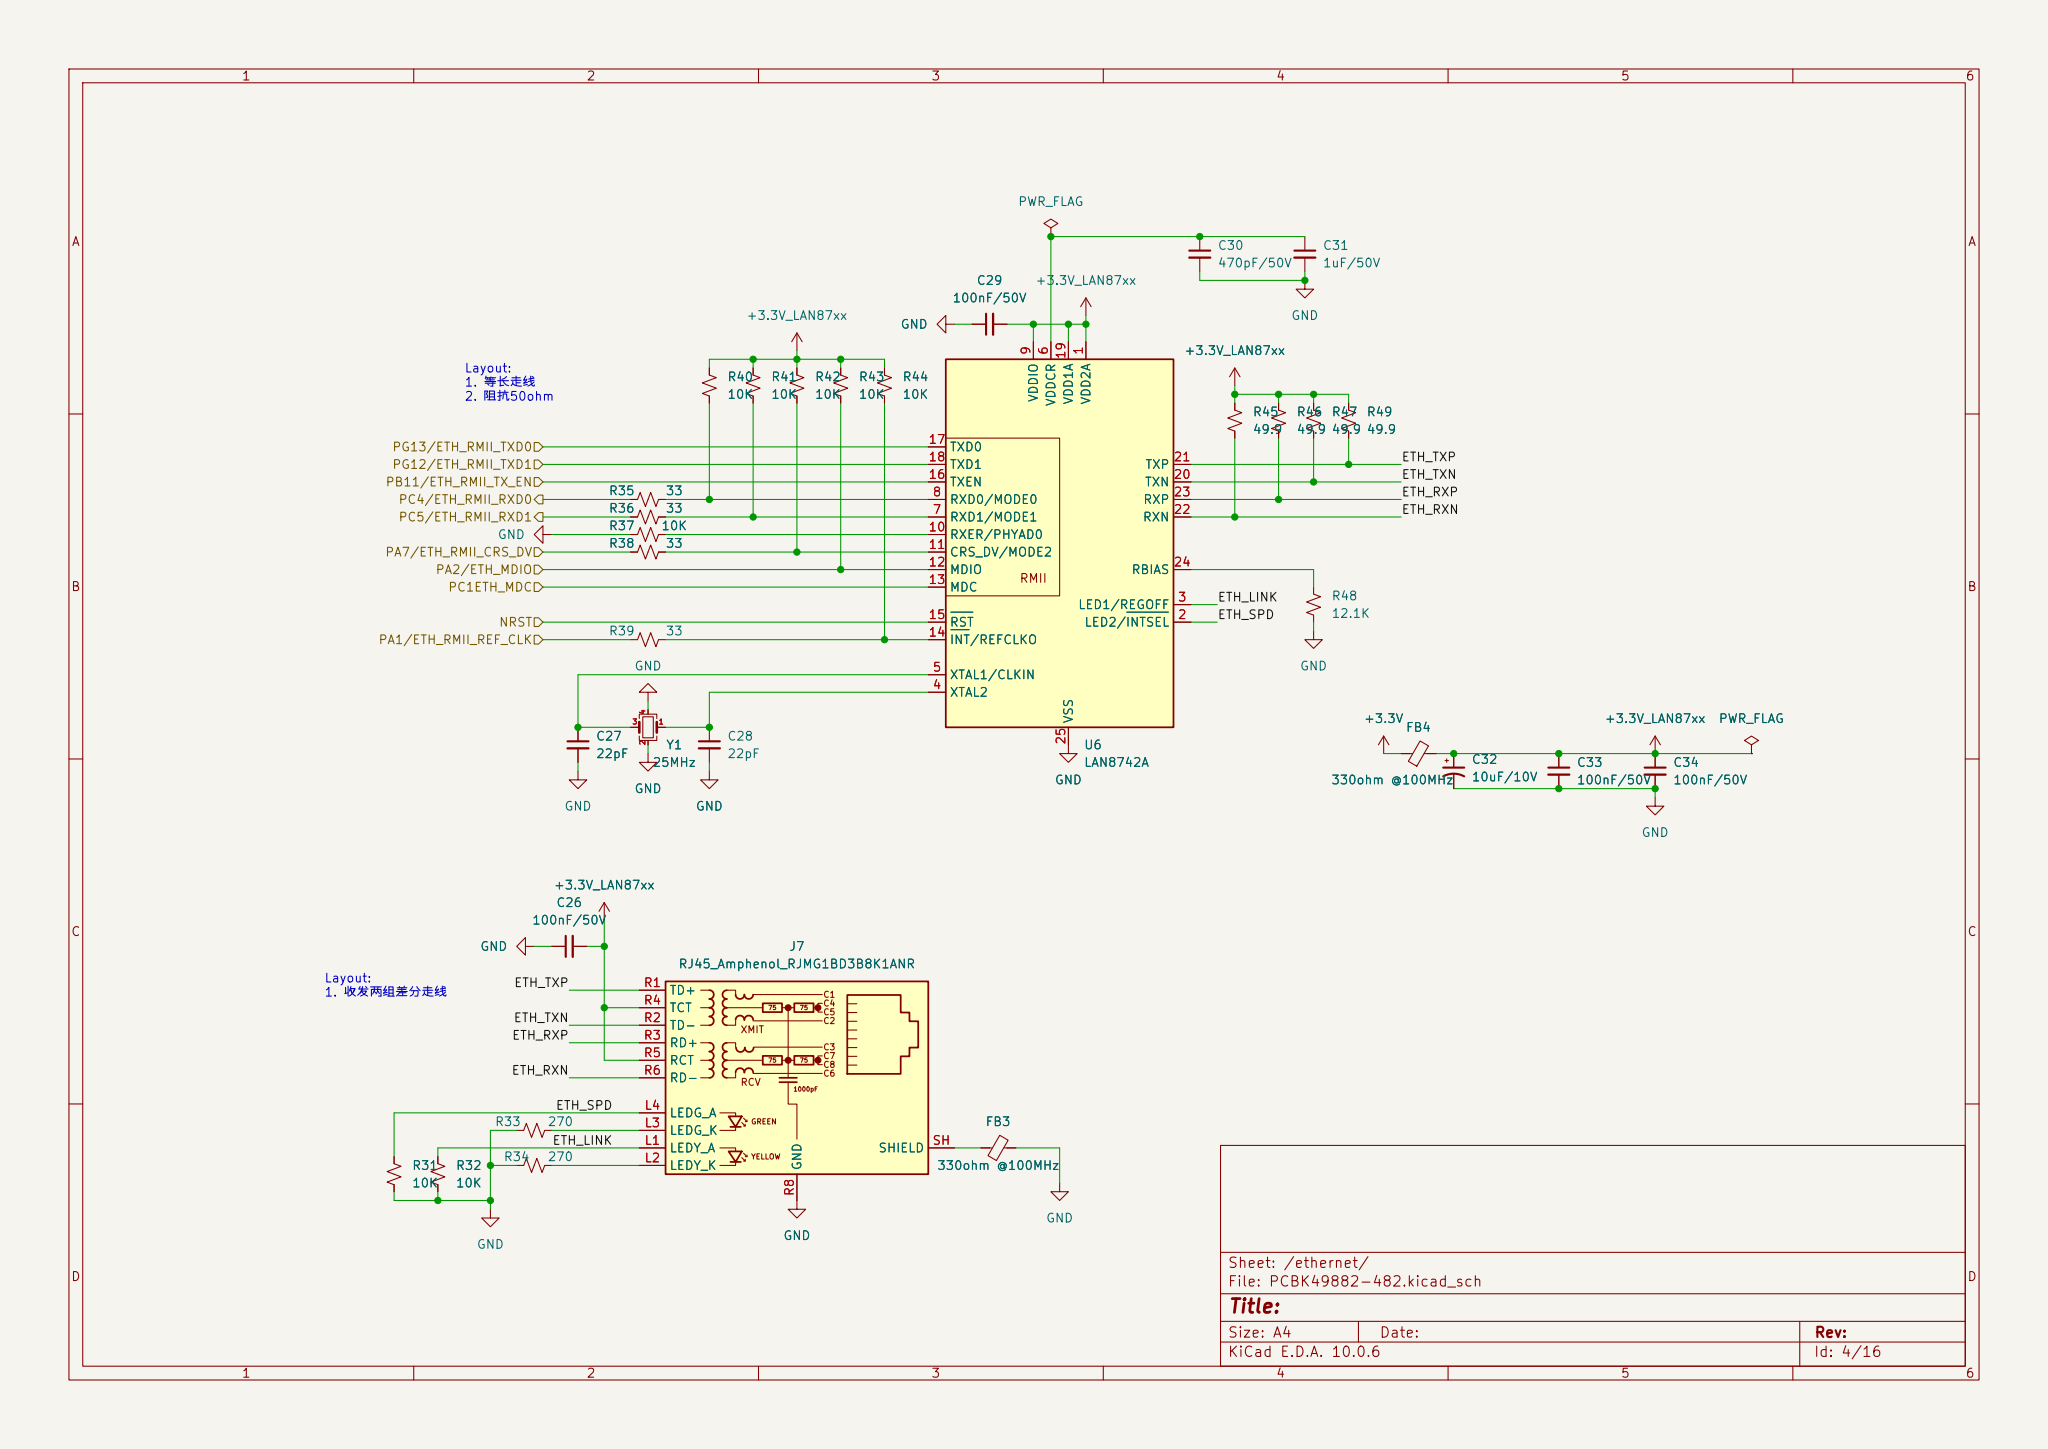Circuit board | KiCad | 536 parts | 438 nets | one sheet of the schematic
Parts on this sheet (reference | value | footprint):
C26 | 100nF/50V | Capacitor_SMD:C_0603_1608Metric
C27 | 22pF | Capacitor_SMD:C_0603_1608Metric
C28 | 22pF | Capacitor_SMD:C_0603_1608Metric
C29 | 100nF/50V | Capacitor_SMD:C_0603_1608Metric
C30 | 470pF/50V | Capacitor_SMD:C_0603_1608Metric
C31 | 1uF/50V | Capacitor_SMD:C_0603_1608Metric
C32 | 10uF/10V | Capacitor_Tantalum_SMD:CP_EIA-3528-21_Kemet-B
C33 | 100nF/50V | Capacitor_SMD:C_0603_1608Metric
C34 | 100nF/50V | Capacitor_SMD:C_0603_1608Metric
FB3
FB4
J7 | RJ45_Amphenol_RJMG1BD3B8K1ANR | Connector_RJ:RJ45_Amphenol_RJMG1BD3B8K1ANR
R31
R32
R33 | 270 | Resistor_SMD:R_0603_1608Metric
R34 | 270 | Resistor_SMD:R_0603_1608Metric
R35 | 33 | Resistor_SMD:R_0603_1608Metric
R36 | 33 | Resistor_SMD:R_0603_1608Metric
R37 | 10K | Resistor_SMD:R_0603_1608Metric
R38 | 33 | Resistor_SMD:R_0603_1608Metric
R39 | 33 | Resistor_SMD:R_0603_1608Metric
R40
R41
R42
R43
R44
R45
R46
R47
R48 | 12.1K | Resistor_SMD:R_0603_1608Metric
R49 | 49.9 | Resistor_SMD:R_0603_1608Metric
U6 | LAN8742A | Package_DFN_QFN:VQFN-24-1EP_4x4mm_P0.5mm_EP2.5x2.5mm
Y1 | 25MHz | Crystal:Crystal_SMD_3225-4Pin_3.2x2.5mm
Nets of these parts (net: part-pin ...):
+3.3V: FB4-1
+3.3V_LAN87xx: C26-2 C29-2 C32-1 C33-1 C34-1 FB4-2 J7-R4 J7-R5 R40-1 R41-1 R42-1 R43-1 R44-1 R45-1 R46-1 R47-1 R49-1 U6-1 U6-9 U6-19
/core_board_b2b/PA1{slash}ETH_RMII_REF_CLK: R39-1
/core_board_b2b/PA2{slash}ETH_MDIO: R43-2 U6-12
/core_board_b2b/PA7{slash}ETH_RMII_CRS_DV: R38-1
/core_board_b2b/PC4{slash}ETH_RMII_RXD0: R35-1
/core_board_b2b/PC5{slash}ETH_RMII_RXD1: R36-1
/ethernet/ETH_LINK: J7-L1 R32-2 U6-3
/ethernet/ETH_RXN: J7-R6 R45-2 U6-22
/ethernet/ETH_RXP: J7-R3 R46-2 U6-23
/ethernet/ETH_SPD: J7-L4 R31-1 U6-2
/ethernet/ETH_TXN: J7-R2 R47-2 U6-20
/ethernet/ETH_TXP: J7-R1 R49-2 U6-21
GND: C26-1 C27-2 C28-2 C29-1 C30-2 C31-2 C32-2 C33-2 C34-2 FB3-2 J7-R8 R31-2 R32-1 R33-1 R34-1 R37-1 R48-2 Y1-2 Y1-4 U6-25
Net-(J7-LEDG_K): J7-L3 R33-2
Net-(J7-LEDY_K): J7-L2 R34-2
Net-(J7-SHIELD): FB3-1 J7-SH
Net-(U6-CRS_DV{slash}MODE2): R38-2 R42-2 U6-11
Net-(U6-RBIAS): R48-1 U6-24
Net-(U6-RXD0{slash}MODE0): R35-2 R40-2 U6-8
Net-(U6-RXD1{slash}MODE1): R36-2 R41-2 U6-7
Net-(U6-RXER{slash}PHYAD0): R37-2 U6-10
Net-(U6-VDDCR): C30-1 C31-1 U6-6
Net-(U6-XTAL1{slash}CLKIN): C27-1 Y1-3 U6-5
Net-(U6-XTAL2): C28-1 Y1-1 U6-4
Net-(U6-~{INT}{slash}REFCLKO): R39-2 R44-2 U6-14
unconnected-(J7-NC-PadR7): J7-R7